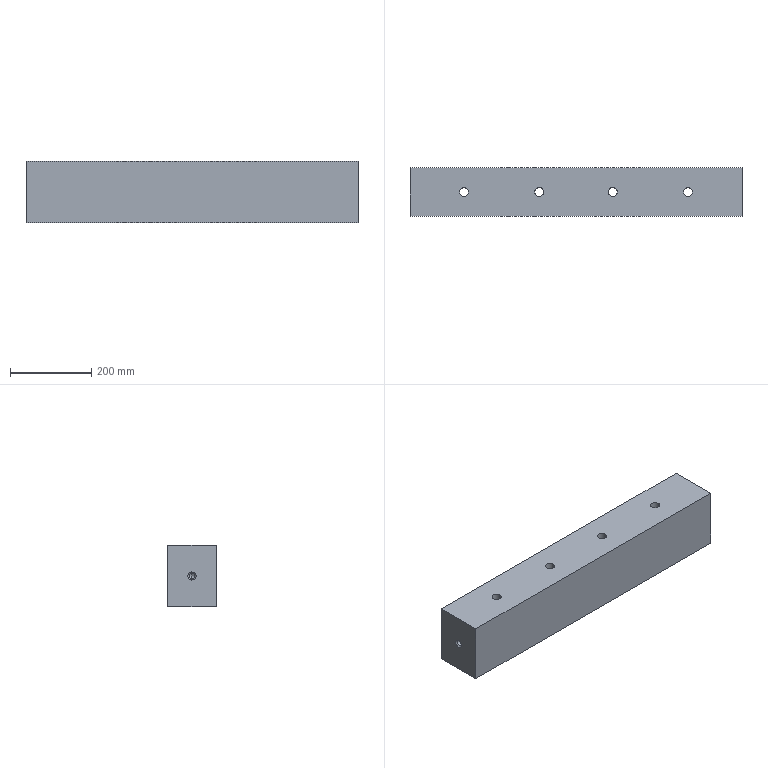Part | Creo | 1 solid | 34 faces | box 815 x 120 x 150 mm | volume 14422262 mm3 | cylinder 16 | cone 12 | plane 6 | commonest cylinder face diameters 22 x8 12 x4 14 x4
STEP:
#1=CARTESIAN_POINT('',(0.,0.,0.));
#2=DIRECTION('',(0.,0.,1.));
#3=DIRECTION('',(1.,0.,0.));
#4=AXIS2_PLACEMENT_3D('',#1,#2,#3);
#5=CARTESIAN_POINT('',(479.101,-434.627,-228.441));
#6=VERTEX_POINT('',#5);
#7=CARTESIAN_POINT('',(479.101,-314.627,-228.441));
#8=VERTEX_POINT('',#7);
#9=CARTESIAN_POINT('',(479.101,-434.627,-228.441));
#10=DIRECTION('',(0.,1.,0.));
#11=VECTOR('',#10,120.);
#12=LINE('',#9,#11);
#13=EDGE_CURVE('',#6,#8,#12,.T.);
#14=ORIENTED_EDGE('',*,*,#13,.T.);
#15=CARTESIAN_POINT('',(479.101,-314.627,-378.441));
#16=VERTEX_POINT('',#15);
#17=CARTESIAN_POINT('',(479.101,-314.627,-228.441));
#18=DIRECTION('',(0.,0.,-1.));
#19=VECTOR('',#18,150.);
#20=LINE('',#17,#19);
#21=EDGE_CURVE('',#8,#16,#20,.T.);
#22=ORIENTED_EDGE('',*,*,#21,.T.);
#23=CARTESIAN_POINT('',(479.101,-434.627,-378.441));
#24=VERTEX_POINT('',#23);
#25=CARTESIAN_POINT('',(479.101,-434.627,-378.441));
#26=DIRECTION('',(0.,1.,0.));
#27=VECTOR('',#26,120.);
#28=LINE('',#25,#27);
#29=EDGE_CURVE('',#24,#16,#28,.T.);
#30=ORIENTED_EDGE('',*,*,#29,.F.);
#31=CARTESIAN_POINT('',(479.101,-434.627,-228.441));
#32=DIRECTION('',(0.,0.,-1.));
#33=VECTOR('',#32,150.);
#34=LINE('',#31,#33);
#35=EDGE_CURVE('',#6,#24,#34,.T.);
#36=ORIENTED_EDGE('',*,*,#35,.F.);
#37=EDGE_LOOP('',(#14,#22,#30,#36));
#38=FACE_OUTER_BOUND('',#37,.F.);
#39=CARTESIAN_POINT('',(479.101,-374.627,-293.441));
#40=VERTEX_POINT('',#39);
#41=CARTESIAN_POINT('',(479.101,-374.627,-313.441));
#42=VERTEX_POINT('',#41);
#43=CARTESIAN_POINT('',(479.101,-374.627,-303.441));
#44=DIRECTION('',(-1.,0.,0.));
#45=DIRECTION('',(0.,0.,1.));
#46=AXIS2_PLACEMENT_3D('',#43,#44,#45);
#47=CIRCLE('',#46,10.);
#48=EDGE_CURVE('',#40,#42,#47,.T.);
#49=ORIENTED_EDGE('',*,*,#48,.F.);
#50=CARTESIAN_POINT('',(479.101,-374.627,-303.441));
#51=DIRECTION('',(-1.,0.,0.));
#52=DIRECTION('',(0.,0.,-1.));
#53=AXIS2_PLACEMENT_3D('',#50,#51,#52);
#54=CIRCLE('',#53,10.);
#55=EDGE_CURVE('',#42,#40,#54,.T.);
#56=ORIENTED_EDGE('',*,*,#55,.F.);
#57=EDGE_LOOP('',(#49,#56));
#58=FACE_BOUND('',#57,.F.);
#59=CARTESIAN_POINT('',(479.101,-314.627,-378.441));
#60=DIRECTION('',(-1.,0.,0.));
#61=DIRECTION('',(0.,0.,1.));
#62=AXIS2_PLACEMENT_3D('',#59,#60,#61);
#63=PLANE('',#62);
#64=ADVANCED_FACE('',(#38,#58),#63,.F.);
#65=CARTESIAN_POINT('',(476.101,-374.627,-296.441));
#66=VERTEX_POINT('',#65);
#67=CARTESIAN_POINT('',(476.101,-374.627,-310.441));
#68=VERTEX_POINT('',#67);
#69=CARTESIAN_POINT('',(476.101,-374.627,-303.441));
#70=DIRECTION('',(-1.,0.,0.));
#71=DIRECTION('',(0.,0.,1.));
#72=AXIS2_PLACEMENT_3D('',#69,#70,#71);
#73=CIRCLE('',#72,7.);
#74=EDGE_CURVE('',#66,#68,#73,.T.);
#75=ORIENTED_EDGE('',*,*,#74,.F.);
#76=CARTESIAN_POINT('',(476.101,-374.627,-296.441));
#77=DIRECTION('',(0.7071,0.,0.7071));
#78=VECTOR('',#77,4.243);
#79=LINE('',#76,#78);
#80=EDGE_CURVE('',#66,#40,#79,.T.);
#81=ORIENTED_EDGE('',*,*,#80,.T.);
#82=ORIENTED_EDGE('',*,*,#48,.T.);
#83=CARTESIAN_POINT('',(476.101,-374.627,-310.441));
#84=DIRECTION('',(0.7071,0.,-0.7071));
#85=VECTOR('',#84,4.243);
#86=LINE('',#83,#85);
#87=EDGE_CURVE('',#68,#42,#86,.T.);
#88=ORIENTED_EDGE('',*,*,#87,.F.);
#89=EDGE_LOOP('',(#75,#81,#82,#88));
#90=FACE_OUTER_BOUND('',#89,.F.);
#91=CARTESIAN_POINT('',(477.601,-374.627,-303.441));
#92=DIRECTION('',(1.,0.,0.));
#93=DIRECTION('',(0.,0.,-1.));
#94=AXIS2_PLACEMENT_3D('',#91,#92,#93);
#95=CONICAL_SURFACE('',#94,8.5,45.);
#96=ADVANCED_FACE('',(#90),#95,.F.);
#97=ORIENTED_EDGE('',*,*,#74,.T.);
#98=CARTESIAN_POINT('',(444.286,-374.627,-310.441));
#99=VERTEX_POINT('',#98);
#100=CARTESIAN_POINT('',(476.101,-374.627,-310.441));
#101=DIRECTION('',(-1.,0.,0.));
#102=VECTOR('',#101,31.815);
#103=LINE('',#100,#102);
#104=EDGE_CURVE('',#68,#99,#103,.T.);
#105=ORIENTED_EDGE('',*,*,#104,.T.);
#106=CARTESIAN_POINT('',(444.286,-374.627,-296.441));
#107=VERTEX_POINT('',#106);
#108=CARTESIAN_POINT('',(444.286,-374.627,-303.441));
#109=DIRECTION('',(1.,0.,0.));
#110=DIRECTION('',(0.,0.,-1.));
#111=AXIS2_PLACEMENT_3D('',#108,#109,#110);
#112=CIRCLE('',#111,7.);
#113=EDGE_CURVE('',#99,#107,#112,.T.);
#114=ORIENTED_EDGE('',*,*,#113,.T.);
#115=CARTESIAN_POINT('',(476.101,-374.627,-296.441));
#116=DIRECTION('',(-1.,0.,0.));
#117=VECTOR('',#116,31.815);
#118=LINE('',#115,#117);
#119=EDGE_CURVE('',#66,#107,#118,.T.);
#120=ORIENTED_EDGE('',*,*,#119,.F.);
#121=EDGE_LOOP('',(#97,#105,#114,#120));
#122=FACE_OUTER_BOUND('',#121,.F.);
#123=CARTESIAN_POINT('',(479.101,-374.627,-303.441));
#124=DIRECTION('',(-1.,0.,0.));
#125=DIRECTION('',(0.,0.,1.));
#126=AXIS2_PLACEMENT_3D('',#123,#124,#125);
#127=CYLINDRICAL_SURFACE('',#126,7.);
#128=ADVANCED_FACE('',(#122),#127,.F.);
#129=CARTESIAN_POINT('',(476.101,-374.627,-303.441));
#130=DIRECTION('',(-1.,0.,0.));
#131=DIRECTION('',(0.,0.,-1.));
#132=AXIS2_PLACEMENT_3D('',#129,#130,#131);
#133=CIRCLE('',#132,7.);
#134=EDGE_CURVE('',#68,#66,#133,.T.);
#135=ORIENTED_EDGE('',*,*,#134,.T.);
#136=ORIENTED_EDGE('',*,*,#119,.T.);
#137=CARTESIAN_POINT('',(444.286,-374.627,-303.441));
#138=DIRECTION('',(1.,0.,0.));
#139=DIRECTION('',(0.,0.,1.));
#140=AXIS2_PLACEMENT_3D('',#137,#138,#139);
#141=CIRCLE('',#140,7.);
#142=EDGE_CURVE('',#107,#99,#141,.T.);
#143=ORIENTED_EDGE('',*,*,#142,.T.);
#144=ORIENTED_EDGE('',*,*,#104,.F.);
#145=EDGE_LOOP('',(#135,#136,#143,#144));
#146=FACE_OUTER_BOUND('',#145,.F.);
#147=CARTESIAN_POINT('',(479.101,-374.627,-303.441));
#148=DIRECTION('',(-1.,0.,0.));
#149=DIRECTION('',(0.,0.,1.));
#150=AXIS2_PLACEMENT_3D('',#147,#148,#149);
#151=CYLINDRICAL_SURFACE('',#150,7.);
#152=ADVANCED_FACE('',(#146),#151,.F.);
#153=ORIENTED_EDGE('',*,*,#134,.F.);
#154=ORIENTED_EDGE('',*,*,#87,.T.);
#155=ORIENTED_EDGE('',*,*,#55,.T.);
#156=ORIENTED_EDGE('',*,*,#80,.F.);
#157=EDGE_LOOP('',(#153,#154,#155,#156));
#158=FACE_OUTER_BOUND('',#157,.F.);
#159=CARTESIAN_POINT('',(477.601,-374.627,-303.441));
#160=DIRECTION('',(1.,0.,0.));
#161=DIRECTION('',(0.,0.,-1.));
#162=AXIS2_PLACEMENT_3D('',#159,#160,#161);
#163=CONICAL_SURFACE('',#162,8.5,45.);
#164=ADVANCED_FACE('',(#158),#163,.F.);
#165=ORIENTED_EDGE('',*,*,#142,.F.);
#166=CARTESIAN_POINT('',(440.08,-374.627,-303.441));
#167=VERTEX_POINT('',#166);
#168=CARTESIAN_POINT('',(440.08,-374.627,-303.441));
#169=DIRECTION('',(0.515,0.,0.8572));
#170=VECTOR('',#169,8.166);
#171=LINE('',#168,#170);
#172=EDGE_CURVE('',#167,#107,#171,.T.);
#173=ORIENTED_EDGE('',*,*,#172,.F.);
#174=CARTESIAN_POINT('',(440.08,-374.627,-303.441));
#175=DIRECTION('',(0.515,0.,-0.8572));
#176=VECTOR('',#175,8.166);
#177=LINE('',#174,#176);
#178=EDGE_CURVE('',#167,#99,#177,.T.);
#179=ORIENTED_EDGE('',*,*,#178,.T.);
#180=EDGE_LOOP('',(#165,#173,#179));
#181=FACE_OUTER_BOUND('',#180,.F.);
#182=CARTESIAN_POINT('',(442.442,-374.627,-303.441));
#183=DIRECTION('',(1.,0.,0.));
#184=DIRECTION('',(0.,0.,-1.));
#185=AXIS2_PLACEMENT_3D('',#182,#183,#184);
#186=CONICAL_SURFACE('',#185,3.931,59.);
#187=ADVANCED_FACE('',(#181),#186,.F.);
#188=ORIENTED_EDGE('',*,*,#113,.F.);
#189=ORIENTED_EDGE('',*,*,#178,.F.);
#190=ORIENTED_EDGE('',*,*,#172,.T.);
#191=EDGE_LOOP('',(#188,#189,#190));
#192=FACE_OUTER_BOUND('',#191,.F.);
#193=CARTESIAN_POINT('',(442.442,-374.627,-303.441));
#194=DIRECTION('',(1.,0.,0.));
#195=DIRECTION('',(0.,0.,-1.));
#196=AXIS2_PLACEMENT_3D('',#193,#194,#195);
#197=CONICAL_SURFACE('',#196,3.931,59.);
#198=ADVANCED_FACE('',(#192),#197,.F.);
#199=ORIENTED_EDGE('',*,*,#13,.F.);
#200=CARTESIAN_POINT('',(-335.899,-434.627,-228.441));
#201=VERTEX_POINT('',#200);
#202=CARTESIAN_POINT('',(-335.899,-434.627,-228.441));
#203=DIRECTION('',(1.,0.,0.));
#204=VECTOR('',#203,815.);
#205=LINE('',#202,#204);
#206=EDGE_CURVE('',#201,#6,#205,.T.);
#207=ORIENTED_EDGE('',*,*,#206,.F.);
#208=CARTESIAN_POINT('',(-335.899,-314.627,-228.441));
#209=VERTEX_POINT('',#208);
#210=CARTESIAN_POINT('',(-335.899,-314.627,-228.441));
#211=DIRECTION('',(0.,-1.,0.));
#212=VECTOR('',#211,120.);
#213=LINE('',#210,#212);
#214=EDGE_CURVE('',#209,#201,#213,.T.);
#215=ORIENTED_EDGE('',*,*,#214,.F.);
#216=CARTESIAN_POINT('',(479.101,-314.627,-228.441));
#217=DIRECTION('',(-1.,0.,0.));
#218=VECTOR('',#217,815.);
#219=LINE('',#216,#218);
#220=EDGE_CURVE('',#8,#209,#219,.T.);
#221=ORIENTED_EDGE('',*,*,#220,.F.);
#222=EDGE_LOOP('',(#199,#207,#215,#221));
#223=FACE_OUTER_BOUND('',#222,.F.);
#224=CARTESIAN_POINT('',(-18.399,-363.627,-228.441));
#225=VERTEX_POINT('',#224);
#226=CARTESIAN_POINT('',(-7.399,-374.627,-228.441));
#227=VERTEX_POINT('',#226);
#228=CARTESIAN_POINT('',(-18.399,-374.627,-228.441));
#229=DIRECTION('',(0.,0.,-1.));
#230=DIRECTION('',(0.,1.,0.));
#231=AXIS2_PLACEMENT_3D('',#228,#229,#230);
#232=CIRCLE('',#231,11.);
#233=EDGE_CURVE('',#225,#227,#232,.T.);
#234=ORIENTED_EDGE('',*,*,#233,.F.);
#235=CARTESIAN_POINT('',(-29.399,-374.627,-228.441));
#236=VERTEX_POINT('',#235);
#237=CARTESIAN_POINT('',(-18.399,-374.627,-228.441));
#238=DIRECTION('',(0.,0.,-1.));
#239=DIRECTION('',(-1.,0.,0.));
#240=AXIS2_PLACEMENT_3D('',#237,#238,#239);
#241=CIRCLE('',#240,11.);
#242=EDGE_CURVE('',#236,#225,#241,.T.);
#243=ORIENTED_EDGE('',*,*,#242,.F.);
#244=CARTESIAN_POINT('',(-18.399,-374.627,-228.441));
#245=DIRECTION('',(0.,0.,-1.));
#246=DIRECTION('',(1.,0.,0.));
#247=AXIS2_PLACEMENT_3D('',#244,#245,#246);
#248=CIRCLE('',#247,11.);
#249=EDGE_CURVE('',#227,#236,#248,.T.);
#250=ORIENTED_EDGE('',*,*,#249,.F.);
#251=EDGE_LOOP('',(#234,#243,#250));
#252=FACE_BOUND('',#251,.F.);
#253=CARTESIAN_POINT('',(346.601,-363.627,-228.441));
#254=VERTEX_POINT('',#253);
#255=CARTESIAN_POINT('',(357.601,-374.627,-228.441));
#256=VERTEX_POINT('',#255);
#257=CARTESIAN_POINT('',(346.601,-374.627,-228.441));
#258=DIRECTION('',(0.,0.,-1.));
#259=DIRECTION('',(0.,1.,0.));
#260=AXIS2_PLACEMENT_3D('',#257,#258,#259);
#261=CIRCLE('',#260,11.);
#262=EDGE_CURVE('',#254,#256,#261,.T.);
#263=ORIENTED_EDGE('',*,*,#262,.F.);
#264=CARTESIAN_POINT('',(335.601,-374.627,-228.441));
#265=VERTEX_POINT('',#264);
#266=CARTESIAN_POINT('',(346.601,-374.627,-228.441));
#267=DIRECTION('',(0.,0.,-1.));
#268=DIRECTION('',(-1.,0.,0.));
#269=AXIS2_PLACEMENT_3D('',#266,#267,#268);
#270=CIRCLE('',#269,11.);
#271=EDGE_CURVE('',#265,#254,#270,.T.);
#272=ORIENTED_EDGE('',*,*,#271,.F.);
#273=CARTESIAN_POINT('',(346.601,-374.627,-228.441));
#274=DIRECTION('',(0.,0.,-1.));
#275=DIRECTION('',(1.,0.,0.));
#276=AXIS2_PLACEMENT_3D('',#273,#274,#275);
#277=CIRCLE('',#276,11.);
#278=EDGE_CURVE('',#256,#265,#277,.T.);
#279=ORIENTED_EDGE('',*,*,#278,.F.);
#280=EDGE_LOOP('',(#263,#272,#279));
#281=FACE_BOUND('',#280,.F.);
#282=CARTESIAN_POINT('',(-203.399,-363.627,-228.441));
#283=VERTEX_POINT('',#282);
#284=CARTESIAN_POINT('',(-192.399,-374.627,-228.441));
#285=VERTEX_POINT('',#284);
#286=CARTESIAN_POINT('',(-203.399,-374.627,-228.441));
#287=DIRECTION('',(0.,0.,-1.));
#288=DIRECTION('',(0.,1.,0.));
#289=AXIS2_PLACEMENT_3D('',#286,#287,#288);
#290=CIRCLE('',#289,11.);
#291=EDGE_CURVE('',#283,#285,#290,.T.);
#292=ORIENTED_EDGE('',*,*,#291,.F.);
#293=CARTESIAN_POINT('',(-214.399,-374.627,-228.441));
#294=VERTEX_POINT('',#293);
#295=CARTESIAN_POINT('',(-203.399,-374.627,-228.441));
#296=DIRECTION('',(0.,0.,-1.));
#297=DIRECTION('',(-1.,0.,0.));
#298=AXIS2_PLACEMENT_3D('',#295,#296,#297);
#299=CIRCLE('',#298,11.);
#300=EDGE_CURVE('',#294,#283,#299,.T.);
#301=ORIENTED_EDGE('',*,*,#300,.F.);
#302=CARTESIAN_POINT('',(-203.399,-374.627,-228.441));
#303=DIRECTION('',(0.,0.,-1.));
#304=DIRECTION('',(1.,0.,0.));
#305=AXIS2_PLACEMENT_3D('',#302,#303,#304);
#306=CIRCLE('',#305,11.);
#307=EDGE_CURVE('',#285,#294,#306,.T.);
#308=ORIENTED_EDGE('',*,*,#307,.F.);
#309=EDGE_LOOP('',(#292,#301,#308));
#310=FACE_BOUND('',#309,.F.);
#311=CARTESIAN_POINT('',(161.601,-363.627,-228.441));
#312=VERTEX_POINT('',#311);
#313=CARTESIAN_POINT('',(172.601,-374.627,-228.441));
#314=VERTEX_POINT('',#313);
#315=CARTESIAN_POINT('',(161.601,-374.627,-228.441));
#316=DIRECTION('',(0.,0.,-1.));
#317=DIRECTION('',(0.,1.,0.));
#318=AXIS2_PLACEMENT_3D('',#315,#316,#317);
#319=CIRCLE('',#318,11.);
#320=EDGE_CURVE('',#312,#314,#319,.T.);
#321=ORIENTED_EDGE('',*,*,#320,.F.);
#322=CARTESIAN_POINT('',(150.601,-374.627,-228.441));
#323=VERTEX_POINT('',#322);
#324=CARTESIAN_POINT('',(161.601,-374.627,-228.441));
#325=DIRECTION('',(0.,0.,-1.));
#326=DIRECTION('',(-1.,0.,0.));
#327=AXIS2_PLACEMENT_3D('',#324,#325,#326);
#328=CIRCLE('',#327,11.);
#329=EDGE_CURVE('',#323,#312,#328,.T.);
#330=ORIENTED_EDGE('',*,*,#329,.F.);
#331=CARTESIAN_POINT('',(161.601,-374.627,-228.441));
#332=DIRECTION('',(0.,0.,-1.));
#333=DIRECTION('',(1.,0.,0.));
#334=AXIS2_PLACEMENT_3D('',#331,#332,#333);
#335=CIRCLE('',#334,11.);
#336=EDGE_CURVE('',#314,#323,#335,.T.);
#337=ORIENTED_EDGE('',*,*,#336,.F.);
#338=EDGE_LOOP('',(#321,#330,#337));
#339=FACE_BOUND('',#338,.F.);
#340=CARTESIAN_POINT('',(464.101,-314.627,-228.441));
#341=DIRECTION('',(0.,0.,1.));
#342=DIRECTION('',(1.,0.,0.));
#343=AXIS2_PLACEMENT_3D('',#340,#341,#342);
#344=PLANE('',#343);
#345=ADVANCED_FACE('',(#223,#252,#281,#310,#339),#344,.T.);
#346=ORIENTED_EDGE('',*,*,#329,.T.);
#347=ORIENTED_EDGE('',*,*,#320,.T.);
#348=CARTESIAN_POINT('',(172.601,-374.627,-378.441));
#349=VERTEX_POINT('',#348);
#350=CARTESIAN_POINT('',(172.601,-374.627,-378.441));
#351=DIRECTION('',(0.,0.,1.));
#352=VECTOR('',#351,150.);
#353=LINE('',#350,#352);
#354=EDGE_CURVE('',#349,#314,#353,.T.);
#355=ORIENTED_EDGE('',*,*,#354,.F.);
#356=CARTESIAN_POINT('',(161.601,-363.627,-378.441));
#357=VERTEX_POINT('',#356);
#358=CARTESIAN_POINT('',(161.601,-374.627,-378.441));
#359=DIRECTION('',(0.,0.,1.));
#360=DIRECTION('',(1.,0.,0.));
#361=AXIS2_PLACEMENT_3D('',#358,#359,#360);
#362=CIRCLE('',#361,11.);
#363=EDGE_CURVE('',#349,#357,#362,.T.);
#364=ORIENTED_EDGE('',*,*,#363,.T.);
#365=CARTESIAN_POINT('',(150.601,-374.627,-378.441));
#366=VERTEX_POINT('',#365);
#367=CARTESIAN_POINT('',(161.601,-374.627,-378.441));
#368=DIRECTION('',(0.,0.,1.));
#369=DIRECTION('',(0.,1.,0.));
#370=AXIS2_PLACEMENT_3D('',#367,#368,#369);
#371=CIRCLE('',#370,11.);
#372=EDGE_CURVE('',#357,#366,#371,.T.);
#373=ORIENTED_EDGE('',*,*,#372,.T.);
#374=CARTESIAN_POINT('',(150.601,-374.627,-378.441));
#375=DIRECTION('',(0.,0.,1.));
#376=VECTOR('',#375,150.);
#377=LINE('',#374,#376);
#378=EDGE_CURVE('',#366,#323,#377,.T.);
#379=ORIENTED_EDGE('',*,*,#378,.T.);
#380=EDGE_LOOP('',(#346,#347,#355,#364,#373,#379));
#381=FACE_OUTER_BOUND('',#380,.F.);
#382=CARTESIAN_POINT('',(161.601,-374.627,-378.441));
#383=DIRECTION('',(0.,0.,1.));
#384=DIRECTION('',(1.,0.,0.));
#385=AXIS2_PLACEMENT_3D('',#382,#383,#384);
#386=CYLINDRICAL_SURFACE('',#385,11.);
#387=ADVANCED_FACE('',(#381),#386,.F.);
#388=ORIENTED_EDGE('',*,*,#336,.T.);
#389=ORIENTED_EDGE('',*,*,#378,.F.);
#390=CARTESIAN_POINT('',(161.601,-385.627,-378.441));
#391=VERTEX_POINT('',#390);
#392=CARTESIAN_POINT('',(161.601,-374.627,-378.441));
#393=DIRECTION('',(0.,0.,1.));
#394=DIRECTION('',(-1.,0.,0.));
#395=AXIS2_PLACEMENT_3D('',#392,#393,#394);
#396=CIRCLE('',#395,11.);
#397=EDGE_CURVE('',#366,#391,#396,.T.);
#398=ORIENTED_EDGE('',*,*,#397,.T.);
#399=CARTESIAN_POINT('',(161.601,-374.627,-378.441));
#400=DIRECTION('',(0.,0.,1.));
#401=DIRECTION('',(0.,-1.,0.));
#402=AXIS2_PLACEMENT_3D('',#399,#400,#401);
#403=CIRCLE('',#402,11.);
#404=EDGE_CURVE('',#391,#349,#403,.T.);
#405=ORIENTED_EDGE('',*,*,#404,.T.);
#406=ORIENTED_EDGE('',*,*,#354,.T.);
#407=EDGE_LOOP('',(#388,#389,#398,#405,#406));
#408=FACE_OUTER_BOUND('',#407,.F.);
#409=CARTESIAN_POINT('',(161.601,-374.627,-378.441));
#410=DIRECTION('',(0.,0.,1.));
#411=DIRECTION('',(1.,0.,0.));
#412=AXIS2_PLACEMENT_3D('',#409,#410,#411);
#413=CYLINDRICAL_SURFACE('',#412,11.);
#414=ADVANCED_FACE('',(#408),#413,.F.);
#415=ORIENTED_EDGE('',*,*,#29,.T.);
#416=CARTESIAN_POINT('',(-335.899,-314.627,-378.441));
#417=VERTEX_POINT('',#416);
#418=CARTESIAN_POINT('',(479.101,-314.627,-378.441));
#419=DIRECTION('',(-1.,0.,0.));
#420=VECTOR('',#419,815.);
#421=LINE('',#418,#420);
#422=EDGE_CURVE('',#16,#417,#421,.T.);
#423=ORIENTED_EDGE('',*,*,#422,.T.);
#424=CARTESIAN_POINT('',(-335.899,-434.627,-378.441));
#425=VERTEX_POINT('',#424);
#426=CARTESIAN_POINT('',(-335.899,-314.627,-378.441));
#427=DIRECTION('',(0.,-1.,0.));
#428=VECTOR('',#427,120.);
#429=LINE('',#426,#428);
#430=EDGE_CURVE('',#417,#425,#429,.T.);
#431=ORIENTED_EDGE('',*,*,#430,.T.);
#432=CARTESIAN_POINT('',(-335.899,-434.627,-378.441));
#433=DIRECTION('',(1.,0.,0.));
#434=VECTOR('',#433,815.);
#435=LINE('',#432,#434);
#436=EDGE_CURVE('',#425,#24,#435,.T.);
#437=ORIENTED_EDGE('',*,*,#436,.T.);
#438=EDGE_LOOP('',(#415,#423,#431,#437));
#439=FACE_OUTER_BOUND('',#438,.F.);
#440=CARTESIAN_POINT('',(-18.399,-363.627,-378.441));
#441=VERTEX_POINT('',#440);
#442=CARTESIAN_POINT('',(-29.399,-374.627,-378.441));
#443=VERTEX_POINT('',#442);
#444=CARTESIAN_POINT('',(-18.399,-374.627,-378.441));
#445=DIRECTION('',(0.,0.,1.));
#446=DIRECTION('',(0.,1.,0.));
#447=AXIS2_PLACEMENT_3D('',#444,#445,#446);
#448=CIRCLE('',#447,11.);
#449=EDGE_CURVE('',#441,#443,#448,.T.);
#450=ORIENTED_EDGE('',*,*,#449,.F.);
#451=CARTESIAN_POINT('',(-7.399,-374.627,-378.441));
#452=VERTEX_POINT('',#451);
#453=CARTESIAN_POINT('',(-18.399,-374.627,-378.441));
#454=DIRECTION('',(0.,0.,1.));
#455=DIRECTION('',(1.,0.,0.));
#456=AXIS2_PLACEMENT_3D('',#453,#454,#455);
#457=CIRCLE('',#456,11.);
#458=EDGE_CURVE('',#452,#441,#457,.T.);
#459=ORIENTED_EDGE('',*,*,#458,.F.);
#460=CARTESIAN_POINT('',(-18.399,-385.627,-378.441));
#461=VERTEX_POINT('',#460);
#462=CARTESIAN_POINT('',(-18.399,-374.627,-378.441));
#463=DIRECTION('',(0.,0.,1.));
#464=DIRECTION('',(0.,-1.,0.));
#465=AXIS2_PLACEMENT_3D('',#462,#463,#464);
#466=CIRCLE('',#465,11.);
#467=EDGE_CURVE('',#461,#452,#466,.T.);
#468=ORIENTED_EDGE('',*,*,#467,.F.);
#469=CARTESIAN_POINT('',(-18.399,-374.627,-378.441));
#470=DIRECTION('',(0.,0.,1.));
#471=DIRECTION('',(-1.,0.,0.));
#472=AXIS2_PLACEMENT_3D('',#469,#470,#471);
#473=CIRCLE('',#472,11.);
#474=EDGE_CURVE('',#443,#461,#473,.T.);
#475=ORIENTED_EDGE('',*,*,#474,.F.);
#476=EDGE_LOOP('',(#450,#459,#468,#475));
#477=FACE_BOUND('',#476,.F.);
#478=CARTESIAN_POINT('',(346.601,-363.627,-378.441));
#479=VERTEX_POINT('',#478);
#480=CARTESIAN_POINT('',(335.601,-374.627,-378.441));
#481=VERTEX_POINT('',#480);
#482=CARTESIAN_POINT('',(346.601,-374.627,-378.441));
#483=DIRECTION('',(0.,0.,1.));
#484=DIRECTION('',(0.,1.,0.));
#485=AXIS2_PLACEMENT_3D('',#482,#483,#484);
#486=CIRCLE('',#485,11.);
#487=EDGE_CURVE('',#479,#481,#486,.T.);
#488=ORIENTED_EDGE('',*,*,#487,.F.);
#489=CARTESIAN_POINT('',(357.601,-374.627,-378.441));
#490=VERTEX_POINT('',#489);
#491=CARTESIAN_POINT('',(346.601,-374.627,-378.441));
#492=DIRECTION('',(0.,0.,1.));
#493=DIRECTION('',(1.,0.,0.));
#494=AXIS2_PLACEMENT_3D('',#491,#492,#493);
#495=CIRCLE('',#494,11.);
#496=EDGE_CURVE('',#490,#479,#495,.T.);
#497=ORIENTED_EDGE('',*,*,#496,.F.);
#498=CARTESIAN_POINT('',(346.601,-385.627,-378.441));
#499=VERTEX_POINT('',#498);
#500=CARTESIAN_POINT('',(346.601,-374.627,-378.441));
#501=DIRECTION('',(0.,0.,1.));
#502=DIRECTION('',(0.,-1.,0.));
#503=AXIS2_PLACEMENT_3D('',#500,#501,#502);
#504=CIRCLE('',#503,11.);
#505=EDGE_CURVE('',#499,#490,#504,.T.);
#506=ORIENTED_EDGE('',*,*,#505,.F.);
#507=CARTESIAN_POINT('',(346.601,-374.627,-378.441));
#508=DIRECTION('',(0.,0.,1.));
#509=DIRECTION('',(-1.,0.,0.));
#510=AXIS2_PLACEMENT_3D('',#507,#508,#509);
#511=CIRCLE('',#510,11.);
#512=EDGE_CURVE('',#481,#499,#511,.T.);
#513=ORIENTED_EDGE('',*,*,#512,.F.);
#514=EDGE_LOOP('',(#488,#497,#506,#513));
#515=FACE_BOUND('',#514,.F.);
#516=CARTESIAN_POINT('',(-203.399,-363.627,-378.441));
#517=VERTEX_POINT('',#516);
#518=CARTESIAN_POINT('',(-214.399,-374.627,-378.441));
#519=VERTEX_POINT('',#518);
#520=CARTESIAN_POINT('',(-203.399,-374.627,-378.441));
#521=DIRECTION('',(0.,0.,1.));
#522=DIRECTION('',(0.,1.,0.));
#523=AXIS2_PLACEMENT_3D('',#520,#521,#522);
#524=CIRCLE('',#523,11.);
#525=EDGE_CURVE('',#517,#519,#524,.T.);
#526=ORIENTED_EDGE('',*,*,#525,.F.);
#527=CARTESIAN_POINT('',(-192.399,-374.627,-378.441));
#528=VERTEX_POINT('',#527);
#529=CARTESIAN_POINT('',(-203.399,-374.627,-378.441));
#530=DIRECTION('',(0.,0.,1.));
#531=DIRECTION('',(1.,0.,0.));
#532=AXIS2_PLACEMENT_3D('',#529,#530,#531);
#533=CIRCLE('',#532,11.);
#534=EDGE_CURVE('',#528,#517,#533,.T.);
#535=ORIENTED_EDGE('',*,*,#534,.F.);
#536=CARTESIAN_POINT('',(-203.399,-385.627,-378.441));
#537=VERTEX_POINT('',#536);
#538=CARTESIAN_POINT('',(-203.399,-374.627,-378.441));
#539=DIRECTION('',(0.,0.,1.));
#540=DIRECTION('',(0.,-1.,0.));
#541=AXIS2_PLACEMENT_3D('',#538,#539,#540);
#542=CIRCLE('',#541,11.);
#543=EDGE_CURVE('',#537,#528,#542,.T.);
#544=ORIENTED_EDGE('',*,*,#543,.F.);
#545=CARTESIAN_POINT('',(-203.399,-374.627,-378.441));
#546=DIRECTION('',(0.,0.,1.));
#547=DIRECTION('',(-1.,0.,0.));
#548=AXIS2_PLACEMENT_3D('',#545,#546,#547);
#549=CIRCLE('',#548,11.);
#550=EDGE_CURVE('',#519,#537,#549,.T.);
#551=ORIENTED_EDGE('',*,*,#550,.F.);
#552=EDGE_LOOP('',(#526,#535,#544,#551));
#553=FACE_BOUND('',#552,.F.);
#554=CARTESIAN_POINT('',(426.101,-368.627,-378.441));
#555=VERTEX_POINT('',#554);
#556=CARTESIAN_POINT('',(420.101,-374.627,-378.441));
#557=VERTEX_POINT('',#556);
#558=CARTESIAN_POINT('',(426.101,-374.627,-378.441));
#559=DIRECTION('',(0.,0.,1.));
#560=DIRECTION('',(0.,1.,0.));
#561=AXIS2_PLACEMENT_3D('',#558,#559,#560);
#562=CIRCLE('',#561,6.);
#563=EDGE_CURVE('',#555,#557,#562,.T.);
#564=ORIENTED_EDGE('',*,*,#563,.F.);
#565=CARTESIAN_POINT('',(432.101,-374.627,-378.441));
#566=VERTEX_POINT('',#565);
#567=CARTESIAN_POINT('',(426.101,-374.627,-378.441));
#568=DIRECTION('',(0.,0.,1.));
#569=DIRECTION('',(1.,0.,0.));
#570=AXIS2_PLACEMENT_3D('',#567,#568,#569);
#571=CIRCLE('',#570,6.);
#572=EDGE_CURVE('',#566,#555,#571,.T.);
#573=ORIENTED_EDGE('',*,*,#572,.F.);
#574=CARTESIAN_POINT('',(426.101,-380.627,-378.441));
#575=VERTEX_POINT('',#574);
#576=CARTESIAN_POINT('',(426.101,-374.627,-378.441));
#577=DIRECTION('',(0.,0.,1.));
#578=DIRECTION('',(0.,-1.,0.));
#579=AXIS2_PLACEMENT_3D('',#576,#577,#578);
#580=CIRCLE('',#579,6.);
#581=EDGE_CURVE('',#575,#566,#580,.T.);
#582=ORIENTED_EDGE('',*,*,#581,.F.);
#583=CARTESIAN_POINT('',(426.101,-374.627,-378.441));
#584=DIRECTION('',(0.,0.,1.));
#585=DIRECTION('',(-1.,0.,0.));
#586=AXIS2_PLACEMENT_3D('',#583,#584,#585);
#587=CIRCLE('',#586,6.);
#588=EDGE_CURVE('',#557,#575,#587,.T.);
#589=ORIENTED_EDGE('',*,*,#588,.F.);
#590=EDGE_LOOP('',(#564,#573,#582,#589));
#591=FACE_BOUND('',#590,.F.);
#592=CARTESIAN_POINT('',(-282.899,-368.627,-378.441));
#593=VERTEX_POINT('',#592);
#594=CARTESIAN_POINT('',(-288.899,-374.627,-378.441));
#595=VERTEX_POINT('',#594);
#596=CARTESIAN_POINT('',(-282.899,-374.627,-378.441));
#597=DIRECTION('',(0.,0.,1.));
#598=DIRECTION('',(0.,1.,0.));
#599=AXIS2_PLACEMENT_3D('',#596,#597,#598);
#600=CIRCLE('',#599,6.);
#601=EDGE_CURVE('',#593,#595,#600,.T.);
#602=ORIENTED_EDGE('',*,*,#601,.F.);
#603=CARTESIAN_POINT('',(-276.899,-374.627,-378.441));
#604=VERTEX_POINT('',#603);
#605=CARTESIAN_POINT('',(-282.899,-374.627,-378.441));
#606=DIRECTION('',(0.,0.,1.));
#607=DIRECTION('',(1.,0.,0.));
#608=AXIS2_PLACEMENT_3D('',#605,#606,#607);
#609=CIRCLE('',#608,6.);
#610=EDGE_CURVE('',#604,#593,#609,.T.);
#611=ORIENTED_EDGE('',*,*,#610,.F.);
#612=CARTESIAN_POINT('',(-282.899,-380.627,-378.441));
#613=VERTEX_POINT('',#612);
#614=CARTESIAN_POINT('',(-282.899,-374.627,-378.441));
#615=DIRECTION('',(0.,0.,1.));
#616=DIRECTION('',(0.,-1.,0.));
#617=AXIS2_PLACEMENT_3D('',#614,#615,#616);
#618=CIRCLE('',#617,6.);
#619=EDGE_CURVE('',#613,#604,#618,.T.);
#620=ORIENTED_EDGE('',*,*,#619,.F.);
#621=CARTESIAN_POINT('',(-282.899,-374.627,-378.441));
#622=DIRECTION('',(0.,0.,1.));
#623=DIRECTION('',(-1.,0.,0.));
#624=AXIS2_PLACEMENT_3D('',#621,#622,#623);
#625=CIRCLE('',#624,6.);
#626=EDGE_CURVE('',#595,#613,#625,.T.);
#627=ORIENTED_EDGE('',*,*,#626,.F.);
#628=EDGE_LOOP('',(#602,#611,#620,#627));
#629=FACE_BOUND('',#628,.F.);
#630=ORIENTED_EDGE('',*,*,#372,.F.);
#631=ORIENTED_EDGE('',*,*,#363,.F.);
#632=ORIENTED_EDGE('',*,*,#404,.F.);
#633=ORIENTED_EDGE('',*,*,#397,.F.);
#634=EDGE_LOOP('',(#630,#631,#632,#633));
#635=FACE_BOUND('',#634,.F.);
#636=CARTESIAN_POINT('',(464.101,-314.627,-378.441));
#637=DIRECTION('',(0.,0.,1.));
#638=DIRECTION('',(1.,0.,0.));
#639=AXIS2_PLACEMENT_3D('',#636,#637,#638);
#640=PLANE('',#639);
#641=ADVANCED_FACE('',(#439,#477,#515,#553,#591,#629,#635),#640,.F.);
#642=ORIENTED_EDGE('',*,*,#242,.T.);
#643=ORIENTED_EDGE('',*,*,#233,.T.);
#644=CARTESIAN_POINT('',(-7.399,-374.627,-378.441));
#645=DIRECTION('',(0.,0.,1.));
#646=VECTOR('',#645,150.);
#647=LINE('',#644,#646);
#648=EDGE_CURVE('',#452,#227,#647,.T.);
#649=ORIENTED_EDGE('',*,*,#648,.F.);
#650=ORIENTED_EDGE('',*,*,#458,.T.);
#651=ORIENTED_EDGE('',*,*,#449,.T.);
#652=CARTESIAN_POINT('',(-29.399,-374.627,-378.441));
#653=DIRECTION('',(0.,0.,1.));
#654=VECTOR('',#653,150.);
#655=LINE('',#652,#654);
#656=EDGE_CURVE('',#443,#236,#655,.T.);
#657=ORIENTED_EDGE('',*,*,#656,.T.);
#658=EDGE_LOOP('',(#642,#643,#649,#650,#651,#657));
#659=FACE_OUTER_BOUND('',#658,.F.);
#660=CARTESIAN_POINT('',(-18.399,-374.627,-378.441));
#661=DIRECTION('',(0.,0.,1.));
#662=DIRECTION('',(1.,0.,0.));
#663=AXIS2_PLACEMENT_3D('',#660,#661,#662);
#664=CYLINDRICAL_SURFACE('',#663,11.);
#665=ADVANCED_FACE('',(#659),#664,.F.);
#666=ORIENTED_EDGE('',*,*,#249,.T.);
#667=ORIENTED_EDGE('',*,*,#656,.F.);
#668=ORIENTED_EDGE('',*,*,#474,.T.);
#669=ORIENTED_EDGE('',*,*,#467,.T.);
#670=ORIENTED_EDGE('',*,*,#648,.T.);
#671=EDGE_LOOP('',(#666,#667,#668,#669,#670));
#672=FACE_OUTER_BOUND('',#671,.F.);
#673=CARTESIAN_POINT('',(-18.399,-374.627,-378.441));
#674=DIRECTION('',(0.,0.,1.));
#675=DIRECTION('',(1.,0.,0.));
#676=AXIS2_PLACEMENT_3D('',#673,#674,#675);
#677=CYLINDRICAL_SURFACE('',#676,11.);
#678=ADVANCED_FACE('',(#672),#677,.F.);
#679=ORIENTED_EDGE('',*,*,#271,.T.);
#680=ORIENTED_EDGE('',*,*,#262,.T.);
#681=CARTESIAN_POINT('',(357.601,-374.627,-378.441));
#682=DIRECTION('',(0.,0.,1.));
#683=VECTOR('',#682,150.);
#684=LINE('',#681,#683);
#685=EDGE_CURVE('',#490,#256,#684,.T.);
#686=ORIENTED_EDGE('',*,*,#685,.F.);
#687=ORIENTED_EDGE('',*,*,#496,.T.);
#688=ORIENTED_EDGE('',*,*,#487,.T.);
#689=CARTESIAN_POINT('',(335.601,-374.627,-378.441));
#690=DIRECTION('',(0.,0.,1.));
#691=VECTOR('',#690,150.);
#692=LINE('',#689,#691);
#693=EDGE_CURVE('',#481,#265,#692,.T.);
#694=ORIENTED_EDGE('',*,*,#693,.T.);
#695=EDGE_LOOP('',(#679,#680,#686,#687,#688,#694));
#696=FACE_OUTER_BOUND('',#695,.F.);
#697=CARTESIAN_POINT('',(346.601,-374.627,-378.441));
#698=DIRECTION('',(0.,0.,1.));
#699=DIRECTION('',(1.,0.,0.));
#700=AXIS2_PLACEMENT_3D('',#697,#698,#699);
#701=CYLINDRICAL_SURFACE('',#700,11.);
#702=ADVANCED_FACE('',(#696),#701,.F.);
#703=ORIENTED_EDGE('',*,*,#278,.T.);
#704=ORIENTED_EDGE('',*,*,#693,.F.);
#705=ORIENTED_EDGE('',*,*,#512,.T.);
#706=ORIENTED_EDGE('',*,*,#505,.T.);
#707=ORIENTED_EDGE('',*,*,#685,.T.);
#708=EDGE_LOOP('',(#703,#704,#705,#706,#707));
#709=FACE_OUTER_BOUND('',#708,.F.);
#710=CARTESIAN_POINT('',(346.601,-374.627,-378.441));
#711=DIRECTION('',(0.,0.,1.));
#712=DIRECTION('',(1.,0.,0.));
#713=AXIS2_PLACEMENT_3D('',#710,#711,#712);
#714=CYLINDRICAL_SURFACE('',#713,11.);
#715=ADVANCED_FACE('',(#709),#714,.F.);
#716=ORIENTED_EDGE('',*,*,#300,.T.);
#717=ORIENTED_EDGE('',*,*,#291,.T.);
#718=CARTESIAN_POINT('',(-192.399,-374.627,-378.441));
#719=DIRECTION('',(0.,0.,1.));
#720=VECTOR('',#719,150.);
#721=LINE('',#718,#720);
#722=EDGE_CURVE('',#528,#285,#721,.T.);
#723=ORIENTED_EDGE('',*,*,#722,.F.);
#724=ORIENTED_EDGE('',*,*,#534,.T.);
#725=ORIENTED_EDGE('',*,*,#525,.T.);
#726=CARTESIAN_POINT('',(-214.399,-374.627,-378.441));
#727=DIRECTION('',(0.,0.,1.));
#728=VECTOR('',#727,150.);
#729=LINE('',#726,#728);
#730=EDGE_CURVE('',#519,#294,#729,.T.);
#731=ORIENTED_EDGE('',*,*,#730,.T.);
#732=EDGE_LOOP('',(#716,#717,#723,#724,#725,#731));
#733=FACE_OUTER_BOUND('',#732,.F.);
#734=CARTESIAN_POINT('',(-203.399,-374.627,-378.441));
#735=DIRECTION('',(0.,0.,1.));
#736=DIRECTION('',(1.,0.,0.));
#737=AXIS2_PLACEMENT_3D('',#734,#735,#736);
#738=CYLINDRICAL_SURFACE('',#737,11.);
#739=ADVANCED_FACE('',(#733),#738,.F.);
#740=ORIENTED_EDGE('',*,*,#307,.T.);
#741=ORIENTED_EDGE('',*,*,#730,.F.);
#742=ORIENTED_EDGE('',*,*,#550,.T.);
#743=ORIENTED_EDGE('',*,*,#543,.T.);
#744=ORIENTED_EDGE('',*,*,#722,.T.);
#745=EDGE_LOOP('',(#740,#741,#742,#743,#744));
#746=FACE_OUTER_BOUND('',#745,.F.);
#747=CARTESIAN_POINT('',(-203.399,-374.627,-378.441));
#748=DIRECTION('',(0.,0.,1.));
#749=DIRECTION('',(1.,0.,0.));
#750=AXIS2_PLACEMENT_3D('',#747,#748,#749);
#751=CYLINDRICAL_SURFACE('',#750,11.);
#752=ADVANCED_FACE('',(#746),#751,.F.);
#753=CARTESIAN_POINT('',(420.101,-374.627,-344.029));
#754=VERTEX_POINT('',#753);
#755=CARTESIAN_POINT('',(426.101,-368.627,-344.029));
#756=VERTEX_POINT('',#755);
#757=CARTESIAN_POINT('',(426.101,-374.627,-344.029));
#758=DIRECTION('',(0.,0.,-1.));
#759=DIRECTION('',(-1.,0.,0.));
#760=AXIS2_PLACEMENT_3D('',#757,#758,#759);
#761=CIRCLE('',#760,6.);
#762=EDGE_CURVE('',#754,#756,#761,.T.);
#763=ORIENTED_EDGE('',*,*,#762,.T.);
#764=CARTESIAN_POINT('',(432.101,-374.627,-344.029));
#765=VERTEX_POINT('',#764);
#766=CARTESIAN_POINT('',(426.101,-374.627,-344.029));
#767=DIRECTION('',(0.,0.,-1.));
#768=DIRECTION('',(0.,1.,0.));
#769=AXIS2_PLACEMENT_3D('',#766,#767,#768);
#770=CIRCLE('',#769,6.);
#771=EDGE_CURVE('',#756,#765,#770,.T.);
#772=ORIENTED_EDGE('',*,*,#771,.T.);
#773=CARTESIAN_POINT('',(432.101,-374.627,-378.441));
#774=DIRECTION('',(0.,0.,1.));
#775=VECTOR('',#774,34.413);
#776=LINE('',#773,#775);
#777=EDGE_CURVE('',#566,#765,#776,.T.);
#778=ORIENTED_EDGE('',*,*,#777,.F.);
#779=ORIENTED_EDGE('',*,*,#572,.T.);
#780=ORIENTED_EDGE('',*,*,#563,.T.);
#781=CARTESIAN_POINT('',(420.101,-374.627,-378.441));
#782=DIRECTION('',(0.,0.,1.));
#783=VECTOR('',#782,34.413);
#784=LINE('',#781,#783);
#785=EDGE_CURVE('',#557,#754,#784,.T.);
#786=ORIENTED_EDGE('',*,*,#785,.T.);
#787=EDGE_LOOP('',(#763,#772,#778,#779,#780,#786));
#788=FACE_OUTER_BOUND('',#787,.F.);
#789=CARTESIAN_POINT('',(426.101,-374.627,-378.441));
#790=DIRECTION('',(0.,0.,1.));
#791=DIRECTION('',(1.,0.,0.));
#792=AXIS2_PLACEMENT_3D('',#789,#790,#791);
#793=CYLINDRICAL_SURFACE('',#792,6.);
#794=ADVANCED_FACE('',(#788),#793,.F.);
#795=ORIENTED_EDGE('',*,*,#771,.F.);
#796=ORIENTED_EDGE('',*,*,#762,.F.);
#797=CARTESIAN_POINT('',(426.101,-374.627,-340.423));
#798=VERTEX_POINT('',#797);
#799=CARTESIAN_POINT('',(426.101,-374.627,-340.423));
#800=DIRECTION('',(-0.8572,0.,-0.515));
#801=VECTOR('',#800,7.);
#802=LINE('',#799,#801);
#803=EDGE_CURVE('',#798,#754,#802,.T.);
#804=ORIENTED_EDGE('',*,*,#803,.F.);
#805=CARTESIAN_POINT('',(426.101,-374.627,-340.423));
#806=DIRECTION('',(0.8572,0.,-0.515));
#807=VECTOR('',#806,7.);
#808=LINE('',#805,#807);
#809=EDGE_CURVE('',#798,#765,#808,.T.);
#810=ORIENTED_EDGE('',*,*,#809,.T.);
#811=EDGE_LOOP('',(#795,#796,#804,#810));
#812=FACE_OUTER_BOUND('',#811,.F.);
#813=CARTESIAN_POINT('',(426.101,-374.627,-342.485));
#814=DIRECTION('',(0.,0.,-1.));
#815=DIRECTION('',(-1.,0.,0.));
#816=AXIS2_PLACEMENT_3D('',#813,#814,#815);
#817=CONICAL_SURFACE('',#816,3.431,59.);
#818=ADVANCED_FACE('',(#812),#817,.F.);
#819=CARTESIAN_POINT('',(426.101,-374.627,-344.029));
#820=DIRECTION('',(0.,0.,-1.));
#821=DIRECTION('',(1.,0.,0.));
#822=AXIS2_PLACEMENT_3D('',#819,#820,#821);
#823=CIRCLE('',#822,6.);
#824=EDGE_CURVE('',#765,#754,#823,.T.);
#825=ORIENTED_EDGE('',*,*,#824,.F.);
#826=ORIENTED_EDGE('',*,*,#809,.F.);
#827=ORIENTED_EDGE('',*,*,#803,.T.);
#828=EDGE_LOOP('',(#825,#826,#827));
#829=FACE_OUTER_BOUND('',#828,.F.);
#830=CARTESIAN_POINT('',(426.101,-374.627,-342.485));
#831=DIRECTION('',(0.,0.,-1.));
#832=DIRECTION('',(-1.,0.,0.));
#833=AXIS2_PLACEMENT_3D('',#830,#831,#832);
#834=CONICAL_SURFACE('',#833,3.431,59.);
#835=ADVANCED_FACE('',(#829),#834,.F.);
#836=ORIENTED_EDGE('',*,*,#824,.T.);
#837=ORIENTED_EDGE('',*,*,#785,.F.);
#838=ORIENTED_EDGE('',*,*,#588,.T.);
#839=ORIENTED_EDGE('',*,*,#581,.T.);
#840=ORIENTED_EDGE('',*,*,#777,.T.);
#841=EDGE_LOOP('',(#836,#837,#838,#839,#840));
#842=FACE_OUTER_BOUND('',#841,.F.);
#843=CARTESIAN_POINT('',(426.101,-374.627,-378.441));
#844=DIRECTION('',(0.,0.,1.));
#845=DIRECTION('',(1.,0.,0.));
#846=AXIS2_PLACEMENT_3D('',#843,#844,#845);
#847=CYLINDRICAL_SURFACE('',#846,6.);
#848=ADVANCED_FACE('',(#842),#847,.F.);
#849=CARTESIAN_POINT('',(-288.899,-374.627,-344.029));
#850=VERTEX_POINT('',#849);
#851=CARTESIAN_POINT('',(-282.899,-368.627,-344.029));
#852=VERTEX_POINT('',#851);
#853=CARTESIAN_POINT('',(-282.899,-374.627,-344.029));
#854=DIRECTION('',(0.,0.,-1.));
#855=DIRECTION('',(-1.,0.,0.));
#856=AXIS2_PLACEMENT_3D('',#853,#854,#855);
#857=CIRCLE('',#856,6.);
#858=EDGE_CURVE('',#850,#852,#857,.T.);
#859=ORIENTED_EDGE('',*,*,#858,.T.);
#860=CARTESIAN_POINT('',(-276.899,-374.627,-344.029));
#861=VERTEX_POINT('',#860);
#862=CARTESIAN_POINT('',(-282.899,-374.627,-344.029));
#863=DIRECTION('',(0.,0.,-1.));
#864=DIRECTION('',(0.,1.,0.));
#865=AXIS2_PLACEMENT_3D('',#862,#863,#864);
#866=CIRCLE('',#865,6.);
#867=EDGE_CURVE('',#852,#861,#866,.T.);
#868=ORIENTED_EDGE('',*,*,#867,.T.);
#869=CARTESIAN_POINT('',(-276.899,-374.627,-378.441));
#870=DIRECTION('',(0.,0.,1.));
#871=VECTOR('',#870,34.413);
#872=LINE('',#869,#871);
#873=EDGE_CURVE('',#604,#861,#872,.T.);
#874=ORIENTED_EDGE('',*,*,#873,.F.);
#875=ORIENTED_EDGE('',*,*,#610,.T.);
#876=ORIENTED_EDGE('',*,*,#601,.T.);
#877=CARTESIAN_POINT('',(-288.899,-374.627,-378.441));
#878=DIRECTION('',(0.,0.,1.));
#879=VECTOR('',#878,34.413);
#880=LINE('',#877,#879);
#881=EDGE_CURVE('',#595,#850,#880,.T.);
#882=ORIENTED_EDGE('',*,*,#881,.T.);
#883=EDGE_LOOP('',(#859,#868,#874,#875,#876,#882));
#884=FACE_OUTER_BOUND('',#883,.F.);
#885=CARTESIAN_POINT('',(-282.899,-374.627,-378.441));
#886=DIRECTION('',(0.,0.,1.));
#887=DIRECTION('',(1.,0.,0.));
#888=AXIS2_PLACEMENT_3D('',#885,#886,#887);
#889=CYLINDRICAL_SURFACE('',#888,6.);
#890=ADVANCED_FACE('',(#884),#889,.F.);
#891=ORIENTED_EDGE('',*,*,#867,.F.);
#892=ORIENTED_EDGE('',*,*,#858,.F.);
#893=CARTESIAN_POINT('',(-282.899,-374.627,-340.423));
#894=VERTEX_POINT('',#893);
#895=CARTESIAN_POINT('',(-282.899,-374.627,-340.423));
#896=DIRECTION('',(-0.8572,0.,-0.515));
#897=VECTOR('',#896,7.);
#898=LINE('',#895,#897);
#899=EDGE_CURVE('',#894,#850,#898,.T.);
#900=ORIENTED_EDGE('',*,*,#899,.F.);
#901=CARTESIAN_POINT('',(-282.899,-374.627,-340.423));
#902=DIRECTION('',(0.8572,0.,-0.515));
#903=VECTOR('',#902,7.);
#904=LINE('',#901,#903);
#905=EDGE_CURVE('',#894,#861,#904,.T.);
#906=ORIENTED_EDGE('',*,*,#905,.T.);
#907=EDGE_LOOP('',(#891,#892,#900,#906));
#908=FACE_OUTER_BOUND('',#907,.F.);
#909=CARTESIAN_POINT('',(-282.899,-374.627,-342.485));
#910=DIRECTION('',(0.,0.,-1.));
#911=DIRECTION('',(-1.,0.,0.));
#912=AXIS2_PLACEMENT_3D('',#909,#910,#911);
#913=CONICAL_SURFACE('',#912,3.431,59.);
#914=ADVANCED_FACE('',(#908),#913,.F.);
#915=CARTESIAN_POINT('',(-282.899,-374.627,-344.029));
#916=DIRECTION('',(0.,0.,-1.));
#917=DIRECTION('',(1.,0.,0.));
#918=AXIS2_PLACEMENT_3D('',#915,#916,#917);
#919=CIRCLE('',#918,6.);
#920=EDGE_CURVE('',#861,#850,#919,.T.);
#921=ORIENTED_EDGE('',*,*,#920,.F.);
#922=ORIENTED_EDGE('',*,*,#905,.F.);
#923=ORIENTED_EDGE('',*,*,#899,.T.);
#924=EDGE_LOOP('',(#921,#922,#923));
#925=FACE_OUTER_BOUND('',#924,.F.);
#926=CARTESIAN_POINT('',(-282.899,-374.627,-342.485));
#927=DIRECTION('',(0.,0.,-1.));
#928=DIRECTION('',(-1.,0.,0.));
#929=AXIS2_PLACEMENT_3D('',#926,#927,#928);
#930=CONICAL_SURFACE('',#929,3.431,59.);
#931=ADVANCED_FACE('',(#925),#930,.F.);
#932=ORIENTED_EDGE('',*,*,#920,.T.);
#933=ORIENTED_EDGE('',*,*,#881,.F.);
#934=ORIENTED_EDGE('',*,*,#626,.T.);
#935=ORIENTED_EDGE('',*,*,#619,.T.);
#936=ORIENTED_EDGE('',*,*,#873,.T.);
#937=EDGE_LOOP('',(#932,#933,#934,#935,#936));
#938=FACE_OUTER_BOUND('',#937,.F.);
#939=CARTESIAN_POINT('',(-282.899,-374.627,-378.441));
#940=DIRECTION('',(0.,0.,1.));
#941=DIRECTION('',(1.,0.,0.));
#942=AXIS2_PLACEMENT_3D('',#939,#940,#941);
#943=CYLINDRICAL_SURFACE('',#942,6.);
#944=ADVANCED_FACE('',(#938),#943,.F.);
#945=ORIENTED_EDGE('',*,*,#220,.T.);
#946=CARTESIAN_POINT('',(-335.899,-314.627,-228.441));
#947=DIRECTION('',(0.,0.,-1.));
#948=VECTOR('',#947,150.);
#949=LINE('',#946,#948);
#950=EDGE_CURVE('',#209,#417,#949,.T.);
#951=ORIENTED_EDGE('',*,*,#950,.T.);
#952=ORIENTED_EDGE('',*,*,#422,.F.);
#953=ORIENTED_EDGE('',*,*,#21,.F.);
#954=EDGE_LOOP('',(#945,#951,#952,#953));
#955=FACE_OUTER_BOUND('',#954,.F.);
#956=CARTESIAN_POINT('',(-335.899,-314.627,-378.441));
#957=DIRECTION('',(0.,-1.,0.));
#958=DIRECTION('',(1.,0.,0.));
#959=AXIS2_PLACEMENT_3D('',#956,#957,#958);
#960=PLANE('',#959);
#961=ADVANCED_FACE('',(#955),#960,.F.);
#962=ORIENTED_EDGE('',*,*,#214,.T.);
#963=CARTESIAN_POINT('',(-335.899,-434.627,-228.441));
#964=DIRECTION('',(0.,0.,-1.));
#965=VECTOR('',#964,150.);
#966=LINE('',#963,#965);
#967=EDGE_CURVE('',#201,#425,#966,.T.);
#968=ORIENTED_EDGE('',*,*,#967,.T.);
#969=ORIENTED_EDGE('',*,*,#430,.F.);
#970=ORIENTED_EDGE('',*,*,#950,.F.);
#971=EDGE_LOOP('',(#962,#968,#969,#970));
#972=FACE_OUTER_BOUND('',#971,.F.);
#973=CARTESIAN_POINT('',(-335.899,-374.627,-313.441));
#974=VERTEX_POINT('',#973);
#975=CARTESIAN_POINT('',(-335.899,-374.627,-293.441));
#976=VERTEX_POINT('',#975);
#977=CARTESIAN_POINT('',(-335.899,-374.627,-303.441));
#978=DIRECTION('',(1.,0.,0.));
#979=DIRECTION('',(0.,0.,-1.));
#980=AXIS2_PLACEMENT_3D('',#977,#978,#979);
#981=CIRCLE('',#980,10.);
#982=EDGE_CURVE('',#974,#976,#981,.T.);
#983=ORIENTED_EDGE('',*,*,#982,.F.);
#984=CARTESIAN_POINT('',(-335.899,-374.627,-303.441));
#985=DIRECTION('',(1.,0.,0.));
#986=DIRECTION('',(0.,0.,1.));
#987=AXIS2_PLACEMENT_3D('',#984,#985,#986);
#988=CIRCLE('',#987,10.);
#989=EDGE_CURVE('',#976,#974,#988,.T.);
#990=ORIENTED_EDGE('',*,*,#989,.F.);
#991=EDGE_LOOP('',(#983,#990));
#992=FACE_BOUND('',#991,.F.);
#993=CARTESIAN_POINT('',(-335.899,-434.627,-378.441));
#994=DIRECTION('',(1.,0.,0.));
#995=DIRECTION('',(0.,0.,-1.));
#996=AXIS2_PLACEMENT_3D('',#993,#994,#995);
#997=PLANE('',#996);
#998=ADVANCED_FACE('',(#972,#992),#997,.F.);
#999=CARTESIAN_POINT('',(-332.899,-374.627,-310.441));
#1000=VERTEX_POINT('',#999);
#1001=CARTESIAN_POINT('',(-332.899,-374.627,-296.441));
#1002=VERTEX_POINT('',#1001);
#1003=CARTESIAN_POINT('',(-332.899,-374.627,-303.441));
#1004=DIRECTION('',(1.,0.,0.));
#1005=DIRECTION('',(0.,0.,-1.));
#1006=AXIS2_PLACEMENT_3D('',#1003,#1004,#1005);
#1007=CIRCLE('',#1006,7.);
#1008=EDGE_CURVE('',#1000,#1002,#1007,.T.);
#1009=ORIENTED_EDGE('',*,*,#1008,.F.);
#1010=CARTESIAN_POINT('',(-332.899,-374.627,-310.441));
#1011=DIRECTION('',(-0.7071,0.,-0.7071));
#1012=VECTOR('',#1011,4.243);
#1013=LINE('',#1010,#1012);
#1014=EDGE_CURVE('',#1000,#974,#1013,.T.);
#1015=ORIENTED_EDGE('',*,*,#1014,.T.);
#1016=ORIENTED_EDGE('',*,*,#982,.T.);
#1017=CARTESIAN_POINT('',(-332.899,-374.627,-296.441));
#1018=DIRECTION('',(-0.7071,0.,0.7071));
#1019=VECTOR('',#1018,4.243);
#1020=LINE('',#1017,#1019);
#1021=EDGE_CURVE('',#1002,#976,#1020,.T.);
#1022=ORIENTED_EDGE('',*,*,#1021,.F.);
#1023=EDGE_LOOP('',(#1009,#1015,#1016,#1022));
#1024=FACE_OUTER_BOUND('',#1023,.F.);
#1025=CARTESIAN_POINT('',(-334.399,-374.627,-303.441));
#1026=DIRECTION('',(-1.,0.,0.));
#1027=DIRECTION('',(0.,0.,1.));
#1028=AXIS2_PLACEMENT_3D('',#1025,#1026,#1027);
#1029=CONICAL_SURFACE('',#1028,8.5,45.);
#1030=ADVANCED_FACE('',(#1024),#1029,.F.);
#1031=ORIENTED_EDGE('',*,*,#1008,.T.);
#1032=CARTESIAN_POINT('',(-301.084,-374.627,-296.441));
#1033=VERTEX_POINT('',#1032);
#1034=CARTESIAN_POINT('',(-332.899,-374.627,-296.441));
#1035=DIRECTION('',(1.,0.,0.));
#1036=VECTOR('',#1035,31.815);
#1037=LINE('',#1034,#1036);
#1038=EDGE_CURVE('',#1002,#1033,#1037,.T.);
#1039=ORIENTED_EDGE('',*,*,#1038,.T.);
#1040=CARTESIAN_POINT('',(-301.084,-374.627,-310.441));
#1041=VERTEX_POINT('',#1040);
#1042=CARTESIAN_POINT('',(-301.084,-374.627,-303.441));
#1043=DIRECTION('',(-1.,0.,0.));
#1044=DIRECTION('',(0.,0.,1.));
#1045=AXIS2_PLACEMENT_3D('',#1042,#1043,#1044);
#1046=CIRCLE('',#1045,7.);
#1047=EDGE_CURVE('',#1033,#1041,#1046,.T.);
#1048=ORIENTED_EDGE('',*,*,#1047,.T.);
#1049=CARTESIAN_POINT('',(-332.899,-374.627,-310.441));
#1050=DIRECTION('',(1.,0.,0.));
#1051=VECTOR('',#1050,31.815);
#1052=LINE('',#1049,#1051);
#1053=EDGE_CURVE('',#1000,#1041,#1052,.T.);
#1054=ORIENTED_EDGE('',*,*,#1053,.F.);
#1055=EDGE_LOOP('',(#1031,#1039,#1048,#1054));
#1056=FACE_OUTER_BOUND('',#1055,.F.);
#1057=CARTESIAN_POINT('',(-335.899,-374.627,-303.441));
#1058=DIRECTION('',(1.,0.,0.));
#1059=DIRECTION('',(0.,0.,-1.));
#1060=AXIS2_PLACEMENT_3D('',#1057,#1058,#1059);
#1061=CYLINDRICAL_SURFACE('',#1060,7.);
#1062=ADVANCED_FACE('',(#1056),#1061,.F.);
#1063=CARTESIAN_POINT('',(-332.899,-374.627,-303.441));
#1064=DIRECTION('',(1.,0.,0.));
#1065=DIRECTION('',(0.,0.,1.));
#1066=AXIS2_PLACEMENT_3D('',#1063,#1064,#1065);
#1067=CIRCLE('',#1066,7.);
#1068=EDGE_CURVE('',#1002,#1000,#1067,.T.);
#1069=ORIENTED_EDGE('',*,*,#1068,.T.);
#1070=ORIENTED_EDGE('',*,*,#1053,.T.);
#1071=CARTESIAN_POINT('',(-301.084,-374.627,-303.441));
#1072=DIRECTION('',(-1.,0.,0.));
#1073=DIRECTION('',(0.,0.,-1.));
#1074=AXIS2_PLACEMENT_3D('',#1071,#1072,#1073);
#1075=CIRCLE('',#1074,7.);
#1076=EDGE_CURVE('',#1041,#1033,#1075,.T.);
#1077=ORIENTED_EDGE('',*,*,#1076,.T.);
#1078=ORIENTED_EDGE('',*,*,#1038,.F.);
#1079=EDGE_LOOP('',(#1069,#1070,#1077,#1078));
#1080=FACE_OUTER_BOUND('',#1079,.F.);
#1081=CARTESIAN_POINT('',(-335.899,-374.627,-303.441));
#1082=DIRECTION('',(1.,0.,0.));
#1083=DIRECTION('',(0.,0.,-1.));
#1084=AXIS2_PLACEMENT_3D('',#1081,#1082,#1083);
#1085=CYLINDRICAL_SURFACE('',#1084,7.);
#1086=ADVANCED_FACE('',(#1080),#1085,.F.);
#1087=ORIENTED_EDGE('',*,*,#1068,.F.);
#1088=ORIENTED_EDGE('',*,*,#1021,.T.);
#1089=ORIENTED_EDGE('',*,*,#989,.T.);
#1090=ORIENTED_EDGE('',*,*,#1014,.F.);
#1091=EDGE_LOOP('',(#1087,#1088,#1089,#1090));
#1092=FACE_OUTER_BOUND('',#1091,.F.);
#1093=CARTESIAN_POINT('',(-334.399,-374.627,-303.441));
#1094=DIRECTION('',(-1.,0.,0.));
#1095=DIRECTION('',(0.,0.,1.));
#1096=AXIS2_PLACEMENT_3D('',#1093,#1094,#1095);
#1097=CONICAL_SURFACE('',#1096,8.5,45.);
#1098=ADVANCED_FACE('',(#1092),#1097,.F.);
#1099=ORIENTED_EDGE('',*,*,#1076,.F.);
#1100=CARTESIAN_POINT('',(-296.878,-374.627,-303.441));
#1101=VERTEX_POINT('',#1100);
#1102=CARTESIAN_POINT('',(-296.878,-374.627,-303.441));
#1103=DIRECTION('',(-0.515,0.,-0.8572));
#1104=VECTOR('',#1103,8.166);
#1105=LINE('',#1102,#1104);
#1106=EDGE_CURVE('',#1101,#1041,#1105,.T.);
#1107=ORIENTED_EDGE('',*,*,#1106,.F.);
#1108=CARTESIAN_POINT('',(-296.878,-374.627,-303.441));
#1109=DIRECTION('',(-0.515,0.,0.8572));
#1110=VECTOR('',#1109,8.166);
#1111=LINE('',#1108,#1110);
#1112=EDGE_CURVE('',#1101,#1033,#1111,.T.);
#1113=ORIENTED_EDGE('',*,*,#1112,.T.);
#1114=EDGE_LOOP('',(#1099,#1107,#1113));
#1115=FACE_OUTER_BOUND('',#1114,.F.);
#1116=CARTESIAN_POINT('',(-299.24,-374.627,-303.441));
#1117=DIRECTION('',(-1.,0.,0.));
#1118=DIRECTION('',(0.,0.,1.));
#1119=AXIS2_PLACEMENT_3D('',#1116,#1117,#1118);
#1120=CONICAL_SURFACE('',#1119,3.931,59.);
#1121=ADVANCED_FACE('',(#1115),#1120,.F.);
#1122=ORIENTED_EDGE('',*,*,#1047,.F.);
#1123=ORIENTED_EDGE('',*,*,#1112,.F.);
#1124=ORIENTED_EDGE('',*,*,#1106,.T.);
#1125=EDGE_LOOP('',(#1122,#1123,#1124));
#1126=FACE_OUTER_BOUND('',#1125,.F.);
#1127=CARTESIAN_POINT('',(-299.24,-374.627,-303.441));
#1128=DIRECTION('',(-1.,0.,0.));
#1129=DIRECTION('',(0.,0.,1.));
#1130=AXIS2_PLACEMENT_3D('',#1127,#1128,#1129);
#1131=CONICAL_SURFACE('',#1130,3.931,59.);
#1132=ADVANCED_FACE('',(#1126),#1131,.F.);
#1133=ORIENTED_EDGE('',*,*,#206,.T.);
#1134=ORIENTED_EDGE('',*,*,#35,.T.);
#1135=ORIENTED_EDGE('',*,*,#436,.F.);
#1136=ORIENTED_EDGE('',*,*,#967,.F.);
#1137=EDGE_LOOP('',(#1133,#1134,#1135,#1136));
#1138=FACE_OUTER_BOUND('',#1137,.F.);
#1139=CARTESIAN_POINT('',(464.101,-434.627,-378.441));
#1140=DIRECTION('',(0.,1.,0.));
#1141=DIRECTION('',(-1.,0.,0.));
#1142=AXIS2_PLACEMENT_3D('',#1139,#1140,#1141);
#1143=PLANE('',#1142);
#1144=ADVANCED_FACE('',(#1138),#1143,.F.);
#1145=CLOSED_SHELL('',(#64,#96,#128,#152,#164,#187,#198,#345,#387,#414,#641,#665,#678,#702,#715,#739,#752,#794,#818,#835,#848,#890,#914,#931,#944,#961,#998,#1030,#1062,#1086,#1098,#1121,#1132,#1144));
#1146=MANIFOLD_SOLID_BREP('',#1145);
#1147=(LENGTH_UNIT()NAMED_UNIT(*)SI_UNIT(.MILLI.,.METRE.));
#1148=UNCERTAINTY_MEASURE_WITH_UNIT(LENGTH_MEASURE(0.08373),#1147,'','');
#1149=(NAMED_UNIT(*)PLANE_ANGLE_UNIT()SI_UNIT($,.RADIAN.));
#1150=PLANE_ANGLE_MEASURE_WITH_UNIT(PLANE_ANGLE_MEASURE(0.01745),#1149);
#1151=(CONVERSION_BASED_UNIT('DEGREE',#1150)NAMED_UNIT(*)PLANE_ANGLE_UNIT());
#1152=(NAMED_UNIT(*)SI_UNIT($,.STERADIAN.)SOLID_ANGLE_UNIT());
#1153=(GEOMETRIC_REPRESENTATION_CONTEXT(3)GLOBAL_UNCERTAINTY_ASSIGNED_CONTEXT((#1148))GLOBAL_UNIT_ASSIGNED_CONTEXT((#1147,#1151,#1152))REPRESENTATION_CONTEXT('',''));
#1154=ADVANCED_BREP_SHAPE_REPRESENTATION('',(#4,#1146),#1153);